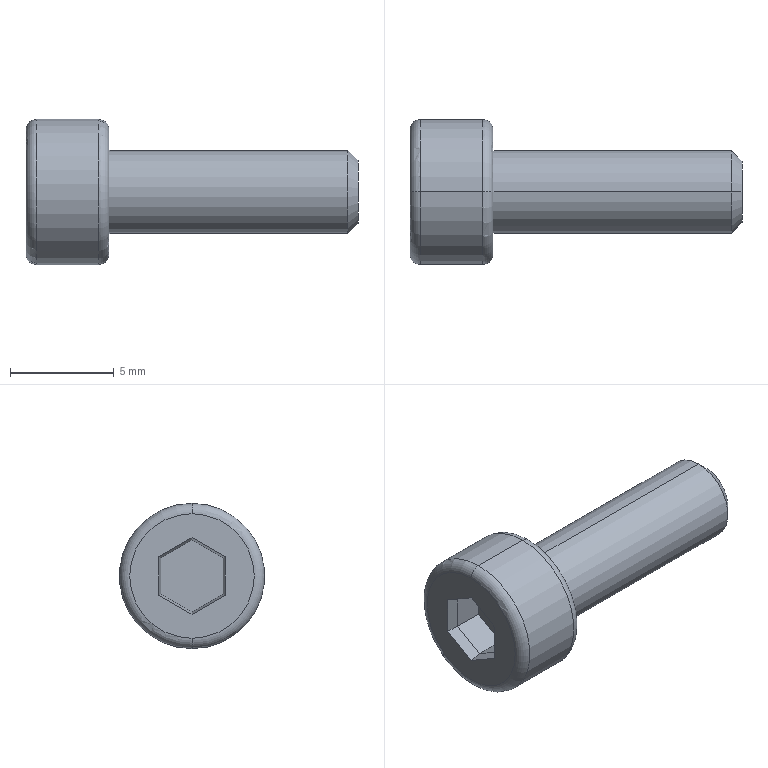Part | SolidWorks | features Chamfer 2, Fillet 1, ICE 1, Revolution 1 | 1 solid | 26 faces | box 16 x 7 x 7 mm | volume 285.121 mm3 | plane 16 | torus 4 | cylinder 4 | cone 2 | commonest cylinder face diameters 4 x2 7 x2
STEP:
#1=CARTESIAN_POINT('',(16.,0.,-1.5));
#2=VERTEX_POINT('',#1);
#3=CARTESIAN_POINT('',(16.,0.,1.5));
#4=VERTEX_POINT('',#3);
#5=CARTESIAN_POINT('',(16.,0.,0.));
#6=DIRECTION('',(1.,0.,0.));
#7=DIRECTION('',(0.,0.,1.));
#8=AXIS2_PLACEMENT_3D('',#5,#6,#7);
#9=CIRCLE('',#8,1.5);
#10=EDGE_CURVE('',#2,#4,#9,.T.);
#11=ORIENTED_EDGE('',*,*,#10,.F.);
#12=CARTESIAN_POINT('',(15.5,0.,-2.));
#13=VERTEX_POINT('',#12);
#14=CARTESIAN_POINT('',(15.5,0.,-2.));
#15=DIRECTION('',(-0.7071,0.,-0.7071));
#16=VECTOR('',#15,1000.);
#17=LINE('',#14,#16);
#18=EDGE_CURVE('',#2,#13,#17,.T.);
#19=ORIENTED_EDGE('',*,*,#18,.T.);
#20=CARTESIAN_POINT('',(15.5,0.,2.));
#21=VERTEX_POINT('',#20);
#22=CARTESIAN_POINT('',(15.5,0.,0.));
#23=DIRECTION('',(-1.,0.,0.));
#24=DIRECTION('',(0.,0.,1.));
#25=AXIS2_PLACEMENT_3D('',#22,#23,#24);
#26=CIRCLE('',#25,2.);
#27=EDGE_CURVE('',#21,#13,#26,.T.);
#28=ORIENTED_EDGE('',*,*,#27,.F.);
#29=CARTESIAN_POINT('',(15.5,0.,2.));
#30=DIRECTION('',(-0.7071,0.,0.7071));
#31=VECTOR('',#30,1000.);
#32=LINE('',#29,#31);
#33=EDGE_CURVE('',#4,#21,#32,.T.);
#34=ORIENTED_EDGE('',*,*,#33,.F.);
#35=EDGE_LOOP('',(#11,#19,#28,#34));
#36=FACE_OUTER_BOUND('',#35,.T.);
#37=CARTESIAN_POINT('',(15.5,0.,0.));
#38=DIRECTION('',(-1.,0.,0.));
#39=DIRECTION('',(0.,0.,1.));
#40=AXIS2_PLACEMENT_3D('',#37,#38,#39);
#41=CONICAL_SURFACE('',#40,2.,0.7854);
#42=ADVANCED_FACE('',(#36),#41,.T.);
#43=CARTESIAN_POINT('',(0.,0.,3.));
#44=VERTEX_POINT('',#43);
#45=CARTESIAN_POINT('',(0.,0.,-3.));
#46=VERTEX_POINT('',#45);
#47=CARTESIAN_POINT('',(0.,0.,0.));
#48=DIRECTION('',(-1.,0.,0.));
#49=DIRECTION('',(0.,0.,-1.));
#50=AXIS2_PLACEMENT_3D('',#47,#48,#49);
#51=CIRCLE('',#50,3.);
#52=EDGE_CURVE('',#44,#46,#51,.T.);
#53=ORIENTED_EDGE('',*,*,#52,.F.);
#54=CARTESIAN_POINT('',(0.5,0.,3.5));
#55=VERTEX_POINT('',#54);
#56=CARTESIAN_POINT('',(0.5,0.,3.));
#57=DIRECTION('',(0.,1.,0.));
#58=DIRECTION('',(0.,0.,1.));
#59=AXIS2_PLACEMENT_3D('',#56,#57,#58);
#60=CIRCLE('',#59,0.5);
#61=EDGE_CURVE('',#44,#55,#60,.T.);
#62=ORIENTED_EDGE('',*,*,#61,.T.);
#63=CARTESIAN_POINT('',(0.5,0.,-3.5));
#64=VERTEX_POINT('',#63);
#65=CARTESIAN_POINT('',(0.5,0.,0.));
#66=DIRECTION('',(1.,0.,0.));
#67=DIRECTION('',(0.,0.,-1.));
#68=AXIS2_PLACEMENT_3D('',#65,#66,#67);
#69=CIRCLE('',#68,3.5);
#70=EDGE_CURVE('',#64,#55,#69,.T.);
#71=ORIENTED_EDGE('',*,*,#70,.F.);
#72=CARTESIAN_POINT('',(0.5,0.,-3.));
#73=DIRECTION('',(0.,-1.,0.));
#74=DIRECTION('',(0.,0.,-1.));
#75=AXIS2_PLACEMENT_3D('',#72,#73,#74);
#76=CIRCLE('',#75,0.5);
#77=EDGE_CURVE('',#46,#64,#76,.T.);
#78=ORIENTED_EDGE('',*,*,#77,.F.);
#79=EDGE_LOOP('',(#53,#62,#71,#78));
#80=FACE_OUTER_BOUND('',#79,.T.);
#81=CARTESIAN_POINT('',(0.5,0.,0.));
#82=DIRECTION('',(1.,0.,0.));
#83=DIRECTION('',(0.,0.,-1.));
#84=AXIS2_PLACEMENT_3D('',#81,#82,#83);
#85=TOROIDAL_SURFACE('',#84,3.,0.5);
#86=ADVANCED_FACE('',(#80),#85,.T.);
#87=CARTESIAN_POINT('',(4.,0.,-3.));
#88=VERTEX_POINT('',#87);
#89=CARTESIAN_POINT('',(4.,0.,3.));
#90=VERTEX_POINT('',#89);
#91=CARTESIAN_POINT('',(4.,0.,0.));
#92=DIRECTION('',(1.,0.,0.));
#93=DIRECTION('',(0.,0.,1.));
#94=AXIS2_PLACEMENT_3D('',#91,#92,#93);
#95=CIRCLE('',#94,3.);
#96=EDGE_CURVE('',#88,#90,#95,.T.);
#97=ORIENTED_EDGE('',*,*,#96,.F.);
#98=CARTESIAN_POINT('',(3.5,0.,-3.5));
#99=VERTEX_POINT('',#98);
#100=CARTESIAN_POINT('',(3.5,0.,-3.));
#101=DIRECTION('',(0.,1.,0.));
#102=DIRECTION('',(0.,0.,1.));
#103=AXIS2_PLACEMENT_3D('',#100,#101,#102);
#104=CIRCLE('',#103,0.5);
#105=EDGE_CURVE('',#88,#99,#104,.T.);
#106=ORIENTED_EDGE('',*,*,#105,.T.);
#107=CARTESIAN_POINT('',(3.5,0.,3.5));
#108=VERTEX_POINT('',#107);
#109=CARTESIAN_POINT('',(3.5,0.,0.));
#110=DIRECTION('',(-1.,0.,0.));
#111=DIRECTION('',(0.,0.,1.));
#112=AXIS2_PLACEMENT_3D('',#109,#110,#111);
#113=CIRCLE('',#112,3.5);
#114=EDGE_CURVE('',#108,#99,#113,.T.);
#115=ORIENTED_EDGE('',*,*,#114,.F.);
#116=CARTESIAN_POINT('',(3.5,0.,3.));
#117=DIRECTION('',(0.,-1.,0.));
#118=DIRECTION('',(0.,0.,-1.));
#119=AXIS2_PLACEMENT_3D('',#116,#117,#118);
#120=CIRCLE('',#119,0.5);
#121=EDGE_CURVE('',#90,#108,#120,.T.);
#122=ORIENTED_EDGE('',*,*,#121,.F.);
#123=EDGE_LOOP('',(#97,#106,#115,#122));
#124=FACE_OUTER_BOUND('',#123,.T.);
#125=CARTESIAN_POINT('',(3.5,0.,0.));
#126=DIRECTION('',(-1.,0.,0.));
#127=DIRECTION('',(0.,0.,1.));
#128=AXIS2_PLACEMENT_3D('',#125,#126,#127);
#129=TOROIDAL_SURFACE('',#128,3.,0.5);
#130=ADVANCED_FACE('',(#124),#129,.T.);
#131=ORIENTED_EDGE('',*,*,#27,.T.);
#132=CARTESIAN_POINT('',(4.,0.,-2.));
#133=VERTEX_POINT('',#132);
#134=CARTESIAN_POINT('',(-4.709,0.,-2.));
#135=DIRECTION('',(-1.,0.,0.));
#136=VECTOR('',#135,1000.);
#137=LINE('',#134,#136);
#138=EDGE_CURVE('',#13,#133,#137,.T.);
#139=ORIENTED_EDGE('',*,*,#138,.T.);
#140=CARTESIAN_POINT('',(4.,0.,2.));
#141=VERTEX_POINT('',#140);
#142=CARTESIAN_POINT('',(4.,0.,0.));
#143=DIRECTION('',(-1.,0.,0.));
#144=DIRECTION('',(0.,0.,1.));
#145=AXIS2_PLACEMENT_3D('',#142,#143,#144);
#146=CIRCLE('',#145,2.);
#147=EDGE_CURVE('',#141,#133,#146,.T.);
#148=ORIENTED_EDGE('',*,*,#147,.F.);
#149=CARTESIAN_POINT('',(-4.709,0.,2.));
#150=DIRECTION('',(-1.,0.,0.));
#151=VECTOR('',#150,1000.);
#152=LINE('',#149,#151);
#153=EDGE_CURVE('',#21,#141,#152,.T.);
#154=ORIENTED_EDGE('',*,*,#153,.F.);
#155=EDGE_LOOP('',(#131,#139,#148,#154));
#156=FACE_OUTER_BOUND('',#155,.T.);
#157=CARTESIAN_POINT('',(-4.709,0.,0.));
#158=DIRECTION('',(-1.,0.,0.));
#159=DIRECTION('',(0.,0.,1.));
#160=AXIS2_PLACEMENT_3D('',#157,#158,#159);
#161=CYLINDRICAL_SURFACE('',#160,2.);
#162=ADVANCED_FACE('',(#156),#161,.T.);
#163=ORIENTED_EDGE('',*,*,#114,.T.);
#164=CARTESIAN_POINT('',(-4.709,0.,-3.5));
#165=DIRECTION('',(-1.,0.,0.));
#166=VECTOR('',#165,1000.);
#167=LINE('',#164,#166);
#168=EDGE_CURVE('',#99,#64,#167,.T.);
#169=ORIENTED_EDGE('',*,*,#168,.T.);
#170=ORIENTED_EDGE('',*,*,#70,.T.);
#171=CARTESIAN_POINT('',(-4.709,0.,3.5));
#172=DIRECTION('',(-1.,0.,0.));
#173=VECTOR('',#172,1000.);
#174=LINE('',#171,#173);
#175=EDGE_CURVE('',#108,#55,#174,.T.);
#176=ORIENTED_EDGE('',*,*,#175,.F.);
#177=EDGE_LOOP('',(#163,#169,#170,#176));
#178=FACE_OUTER_BOUND('',#177,.T.);
#179=CARTESIAN_POINT('',(-4.709,0.,0.));
#180=DIRECTION('',(-1.,0.,0.));
#181=DIRECTION('',(0.,0.,1.));
#182=AXIS2_PLACEMENT_3D('',#179,#180,#181);
#183=CYLINDRICAL_SURFACE('',#182,3.5);
#184=ADVANCED_FACE('',(#178),#183,.T.);
#185=CARTESIAN_POINT('',(0.,-1.6,0.9238));
#186=VERTEX_POINT('',#185);
#187=CARTESIAN_POINT('',(0.,-1.6,-0.9238));
#188=VERTEX_POINT('',#187);
#189=CARTESIAN_POINT('',(0.,-1.6,0.));
#190=DIRECTION('',(0.,0.,-1.));
#191=VECTOR('',#190,1000.);
#192=LINE('',#189,#191);
#193=EDGE_CURVE('',#186,#188,#192,.T.);
#194=ORIENTED_EDGE('',*,*,#193,.T.);
#195=CARTESIAN_POINT('',(0.,0.,-1.848));
#196=VERTEX_POINT('',#195);
#197=CARTESIAN_POINT('',(0.,-0.8,-1.386));
#198=DIRECTION('',(0.,0.866,-0.5));
#199=VECTOR('',#198,1000.);
#200=LINE('',#197,#199);
#201=EDGE_CURVE('',#188,#196,#200,.T.);
#202=ORIENTED_EDGE('',*,*,#201,.T.);
#203=CARTESIAN_POINT('',(0.,1.6,-0.9238));
#204=VERTEX_POINT('',#203);
#205=CARTESIAN_POINT('',(0.,0.8,-1.386));
#206=DIRECTION('',(0.,0.866,0.5));
#207=VECTOR('',#206,1000.);
#208=LINE('',#205,#207);
#209=EDGE_CURVE('',#196,#204,#208,.T.);
#210=ORIENTED_EDGE('',*,*,#209,.T.);
#211=CARTESIAN_POINT('',(0.,1.6,0.9238));
#212=VERTEX_POINT('',#211);
#213=CARTESIAN_POINT('',(0.,1.6,0.));
#214=DIRECTION('',(0.,0.,1.));
#215=VECTOR('',#214,1000.);
#216=LINE('',#213,#215);
#217=EDGE_CURVE('',#204,#212,#216,.T.);
#218=ORIENTED_EDGE('',*,*,#217,.T.);
#219=CARTESIAN_POINT('',(0.,0.,1.848));
#220=VERTEX_POINT('',#219);
#221=CARTESIAN_POINT('',(0.,0.8,1.386));
#222=DIRECTION('',(0.,-0.866,0.5));
#223=VECTOR('',#222,1000.);
#224=LINE('',#221,#223);
#225=EDGE_CURVE('',#212,#220,#224,.T.);
#226=ORIENTED_EDGE('',*,*,#225,.T.);
#227=CARTESIAN_POINT('',(0.,-0.8,1.386));
#228=DIRECTION('',(0.,-0.866,-0.5));
#229=VECTOR('',#228,1000.);
#230=LINE('',#227,#229);
#231=EDGE_CURVE('',#220,#186,#230,.T.);
#232=ORIENTED_EDGE('',*,*,#231,.T.);
#233=EDGE_LOOP('',(#194,#202,#210,#218,#226,#232));
#234=FACE_BOUND('',#233,.T.);
#235=CARTESIAN_POINT('',(0.,0.,0.));
#236=DIRECTION('',(-1.,0.,0.));
#237=DIRECTION('',(0.,0.,-1.));
#238=AXIS2_PLACEMENT_3D('',#235,#236,#237);
#239=CIRCLE('',#238,3.);
#240=EDGE_CURVE('',#46,#44,#239,.T.);
#241=ORIENTED_EDGE('',*,*,#240,.T.);
#242=ORIENTED_EDGE('',*,*,#52,.T.);
#243=EDGE_LOOP('',(#241,#242));
#244=FACE_OUTER_BOUND('',#243,.T.);
#245=CARTESIAN_POINT('',(0.,0.,0.));
#246=DIRECTION('',(1.,0.,0.));
#247=DIRECTION('',(0.,0.,-1.));
#248=AXIS2_PLACEMENT_3D('',#245,#246,#247);
#249=PLANE('',#248);
#250=ADVANCED_FACE('',(#234,#244),#249,.F.);
#251=ORIENTED_EDGE('',*,*,#168,.F.);
#252=CARTESIAN_POINT('',(3.5,0.,0.));
#253=DIRECTION('',(-1.,0.,0.));
#254=DIRECTION('',(0.,0.,1.));
#255=AXIS2_PLACEMENT_3D('',#252,#253,#254);
#256=CIRCLE('',#255,3.5);
#257=EDGE_CURVE('',#99,#108,#256,.T.);
#258=ORIENTED_EDGE('',*,*,#257,.T.);
#259=ORIENTED_EDGE('',*,*,#175,.T.);
#260=CARTESIAN_POINT('',(0.5,0.,0.));
#261=DIRECTION('',(1.,0.,0.));
#262=DIRECTION('',(0.,0.,-1.));
#263=AXIS2_PLACEMENT_3D('',#260,#261,#262);
#264=CIRCLE('',#263,3.5);
#265=EDGE_CURVE('',#55,#64,#264,.T.);
#266=ORIENTED_EDGE('',*,*,#265,.T.);
#267=EDGE_LOOP('',(#251,#258,#259,#266));
#268=FACE_OUTER_BOUND('',#267,.T.);
#269=CARTESIAN_POINT('',(-4.709,0.,0.));
#270=DIRECTION('',(-1.,0.,0.));
#271=DIRECTION('',(0.,0.,1.));
#272=AXIS2_PLACEMENT_3D('',#269,#270,#271);
#273=CYLINDRICAL_SURFACE('',#272,3.5);
#274=ADVANCED_FACE('',(#268),#273,.T.);
#275=CARTESIAN_POINT('',(4.,0.,0.));
#276=DIRECTION('',(1.,0.,0.));
#277=DIRECTION('',(0.,0.,1.));
#278=AXIS2_PLACEMENT_3D('',#275,#276,#277);
#279=CIRCLE('',#278,3.);
#280=EDGE_CURVE('',#90,#88,#279,.T.);
#281=ORIENTED_EDGE('',*,*,#280,.T.);
#282=ORIENTED_EDGE('',*,*,#96,.T.);
#283=EDGE_LOOP('',(#281,#282));
#284=FACE_OUTER_BOUND('',#283,.T.);
#285=ORIENTED_EDGE('',*,*,#147,.T.);
#286=CARTESIAN_POINT('',(4.,0.,0.));
#287=DIRECTION('',(-1.,0.,0.));
#288=DIRECTION('',(0.,0.,1.));
#289=AXIS2_PLACEMENT_3D('',#286,#287,#288);
#290=CIRCLE('',#289,2.);
#291=EDGE_CURVE('',#133,#141,#290,.T.);
#292=ORIENTED_EDGE('',*,*,#291,.T.);
#293=EDGE_LOOP('',(#285,#292));
#294=FACE_BOUND('',#293,.T.);
#295=CARTESIAN_POINT('',(4.,3.5,0.));
#296=DIRECTION('',(-1.,0.,0.));
#297=DIRECTION('',(0.,0.,1.));
#298=AXIS2_PLACEMENT_3D('',#295,#296,#297);
#299=PLANE('',#298);
#300=ADVANCED_FACE('',(#284,#294),#299,.F.);
#301=ORIENTED_EDGE('',*,*,#138,.F.);
#302=CARTESIAN_POINT('',(15.5,0.,0.));
#303=DIRECTION('',(-1.,0.,0.));
#304=DIRECTION('',(0.,0.,1.));
#305=AXIS2_PLACEMENT_3D('',#302,#303,#304);
#306=CIRCLE('',#305,2.);
#307=EDGE_CURVE('',#13,#21,#306,.T.);
#308=ORIENTED_EDGE('',*,*,#307,.T.);
#309=ORIENTED_EDGE('',*,*,#153,.T.);
#310=ORIENTED_EDGE('',*,*,#291,.F.);
#311=EDGE_LOOP('',(#301,#308,#309,#310));
#312=FACE_OUTER_BOUND('',#311,.T.);
#313=CARTESIAN_POINT('',(-4.709,0.,0.));
#314=DIRECTION('',(-1.,0.,0.));
#315=DIRECTION('',(0.,0.,1.));
#316=AXIS2_PLACEMENT_3D('',#313,#314,#315);
#317=CYLINDRICAL_SURFACE('',#316,2.);
#318=ADVANCED_FACE('',(#312),#317,.T.);
#319=CARTESIAN_POINT('',(16.,0.,0.));
#320=DIRECTION('',(1.,0.,0.));
#321=DIRECTION('',(0.,0.,1.));
#322=AXIS2_PLACEMENT_3D('',#319,#320,#321);
#323=CIRCLE('',#322,1.5);
#324=EDGE_CURVE('',#4,#2,#323,.T.);
#325=ORIENTED_EDGE('',*,*,#324,.T.);
#326=ORIENTED_EDGE('',*,*,#10,.T.);
#327=EDGE_LOOP('',(#325,#326));
#328=FACE_OUTER_BOUND('',#327,.T.);
#329=CARTESIAN_POINT('',(16.,2.,0.));
#330=DIRECTION('',(-1.,0.,0.));
#331=DIRECTION('',(0.,0.,1.));
#332=AXIS2_PLACEMENT_3D('',#329,#330,#331);
#333=PLANE('',#332);
#334=ADVANCED_FACE('',(#328),#333,.F.);
#335=CARTESIAN_POINT('',(2.,1.5,-0.866));
#336=VERTEX_POINT('',#335);
#337=CARTESIAN_POINT('',(0.5671,1.5,-0.866));
#338=VERTEX_POINT('',#337);
#339=CARTESIAN_POINT('',(2.,1.5,-0.866));
#340=DIRECTION('',(-1.,0.,0.));
#341=VECTOR('',#340,1000.);
#342=LINE('',#339,#341);
#343=EDGE_CURVE('',#336,#338,#342,.T.);
#344=ORIENTED_EDGE('',*,*,#343,.T.);
#345=CARTESIAN_POINT('',(0.5671,0.,-1.732));
#346=VERTEX_POINT('',#345);
#347=CARTESIAN_POINT('',(0.5671,1.5,-0.866));
#348=DIRECTION('',(0.,-0.866,-0.5));
#349=VECTOR('',#348,1000.);
#350=LINE('',#347,#349);
#351=EDGE_CURVE('',#338,#346,#350,.T.);
#352=ORIENTED_EDGE('',*,*,#351,.T.);
#353=CARTESIAN_POINT('',(2.,0.,-1.732));
#354=VERTEX_POINT('',#353);
#355=CARTESIAN_POINT('',(2.,0.,-1.732));
#356=DIRECTION('',(-1.,0.,0.));
#357=VECTOR('',#356,1000.);
#358=LINE('',#355,#357);
#359=EDGE_CURVE('',#354,#346,#358,.T.);
#360=ORIENTED_EDGE('',*,*,#359,.F.);
#361=CARTESIAN_POINT('',(2.,1.5,-0.866));
#362=DIRECTION('',(0.,-0.866,-0.5));
#363=VECTOR('',#362,1000.);
#364=LINE('',#361,#363);
#365=EDGE_CURVE('',#336,#354,#364,.T.);
#366=ORIENTED_EDGE('',*,*,#365,.F.);
#367=EDGE_LOOP('',(#344,#352,#360,#366));
#368=FACE_OUTER_BOUND('',#367,.T.);
#369=CARTESIAN_POINT('',(2.,1.5,-0.866));
#370=DIRECTION('',(0.,0.5,-0.866));
#371=DIRECTION('',(0.,0.866,0.5));
#372=AXIS2_PLACEMENT_3D('',#369,#370,#371);
#373=PLANE('',#372);
#374=ADVANCED_FACE('',(#368),#373,.F.);
#375=CARTESIAN_POINT('',(2.,1.5,0.866));
#376=VERTEX_POINT('',#375);
#377=CARTESIAN_POINT('',(0.5671,1.5,0.866));
#378=VERTEX_POINT('',#377);
#379=CARTESIAN_POINT('',(2.,1.5,0.866));
#380=DIRECTION('',(-1.,0.,0.));
#381=VECTOR('',#380,1000.);
#382=LINE('',#379,#381);
#383=EDGE_CURVE('',#376,#378,#382,.T.);
#384=ORIENTED_EDGE('',*,*,#383,.T.);
#385=CARTESIAN_POINT('',(0.5671,1.5,0.866));
#386=DIRECTION('',(0.,0.,-1.));
#387=VECTOR('',#386,1000.);
#388=LINE('',#385,#387);
#389=EDGE_CURVE('',#378,#338,#388,.T.);
#390=ORIENTED_EDGE('',*,*,#389,.T.);
#391=ORIENTED_EDGE('',*,*,#343,.F.);
#392=CARTESIAN_POINT('',(2.,1.5,0.866));
#393=DIRECTION('',(0.,0.,-1.));
#394=VECTOR('',#393,1000.);
#395=LINE('',#392,#394);
#396=EDGE_CURVE('',#376,#336,#395,.T.);
#397=ORIENTED_EDGE('',*,*,#396,.F.);
#398=EDGE_LOOP('',(#384,#390,#391,#397));
#399=FACE_OUTER_BOUND('',#398,.T.);
#400=CARTESIAN_POINT('',(2.,1.5,0.866));
#401=DIRECTION('',(0.,1.,0.));
#402=DIRECTION('',(0.,0.,1.));
#403=AXIS2_PLACEMENT_3D('',#400,#401,#402);
#404=PLANE('',#403);
#405=ADVANCED_FACE('',(#399),#404,.F.);
#406=CARTESIAN_POINT('',(2.,0.,1.732));
#407=VERTEX_POINT('',#406);
#408=CARTESIAN_POINT('',(0.5671,0.,1.732));
#409=VERTEX_POINT('',#408);
#410=CARTESIAN_POINT('',(2.,0.,1.732));
#411=DIRECTION('',(-1.,0.,0.));
#412=VECTOR('',#411,1000.);
#413=LINE('',#410,#412);
#414=EDGE_CURVE('',#407,#409,#413,.T.);
#415=ORIENTED_EDGE('',*,*,#414,.T.);
#416=CARTESIAN_POINT('',(0.5671,0.,1.732));
#417=DIRECTION('',(0.,0.866,-0.5));
#418=VECTOR('',#417,1000.);
#419=LINE('',#416,#418);
#420=EDGE_CURVE('',#409,#378,#419,.T.);
#421=ORIENTED_EDGE('',*,*,#420,.T.);
#422=ORIENTED_EDGE('',*,*,#383,.F.);
#423=CARTESIAN_POINT('',(2.,0.,1.732));
#424=DIRECTION('',(0.,0.866,-0.5));
#425=VECTOR('',#424,1000.);
#426=LINE('',#423,#425);
#427=EDGE_CURVE('',#407,#376,#426,.T.);
#428=ORIENTED_EDGE('',*,*,#427,.F.);
#429=EDGE_LOOP('',(#415,#421,#422,#428));
#430=FACE_OUTER_BOUND('',#429,.T.);
#431=CARTESIAN_POINT('',(2.,0.,1.732));
#432=DIRECTION('',(0.,0.5,0.866));
#433=DIRECTION('',(0.,-0.866,0.5));
#434=AXIS2_PLACEMENT_3D('',#431,#432,#433);
#435=PLANE('',#434);
#436=ADVANCED_FACE('',(#430),#435,.F.);
#437=CARTESIAN_POINT('',(2.,-1.5,0.866));
#438=VERTEX_POINT('',#437);
#439=CARTESIAN_POINT('',(0.5671,-1.5,0.866));
#440=VERTEX_POINT('',#439);
#441=CARTESIAN_POINT('',(2.,-1.5,0.866));
#442=DIRECTION('',(-1.,0.,0.));
#443=VECTOR('',#442,1000.);
#444=LINE('',#441,#443);
#445=EDGE_CURVE('',#438,#440,#444,.T.);
#446=ORIENTED_EDGE('',*,*,#445,.T.);
#447=CARTESIAN_POINT('',(0.5671,-1.5,0.866));
#448=DIRECTION('',(0.,0.866,0.5));
#449=VECTOR('',#448,1000.);
#450=LINE('',#447,#449);
#451=EDGE_CURVE('',#440,#409,#450,.T.);
#452=ORIENTED_EDGE('',*,*,#451,.T.);
#453=ORIENTED_EDGE('',*,*,#414,.F.);
#454=CARTESIAN_POINT('',(2.,-1.5,0.866));
#455=DIRECTION('',(0.,0.866,0.5));
#456=VECTOR('',#455,1000.);
#457=LINE('',#454,#456);
#458=EDGE_CURVE('',#438,#407,#457,.T.);
#459=ORIENTED_EDGE('',*,*,#458,.F.);
#460=EDGE_LOOP('',(#446,#452,#453,#459));
#461=FACE_OUTER_BOUND('',#460,.T.);
#462=CARTESIAN_POINT('',(2.,-1.5,0.866));
#463=DIRECTION('',(0.,-0.5,0.866));
#464=DIRECTION('',(0.,-0.866,-0.5));
#465=AXIS2_PLACEMENT_3D('',#462,#463,#464);
#466=PLANE('',#465);
#467=ADVANCED_FACE('',(#461),#466,.F.);
#468=CARTESIAN_POINT('',(2.,-1.5,-0.866));
#469=VERTEX_POINT('',#468);
#470=CARTESIAN_POINT('',(0.5671,-1.5,-0.866));
#471=VERTEX_POINT('',#470);
#472=CARTESIAN_POINT('',(2.,-1.5,-0.866));
#473=DIRECTION('',(-1.,0.,0.));
#474=VECTOR('',#473,1000.);
#475=LINE('',#472,#474);
#476=EDGE_CURVE('',#469,#471,#475,.T.);
#477=ORIENTED_EDGE('',*,*,#476,.T.);
#478=CARTESIAN_POINT('',(0.5671,-1.5,-0.866));
#479=DIRECTION('',(0.,0.,1.));
#480=VECTOR('',#479,1000.);
#481=LINE('',#478,#480);
#482=EDGE_CURVE('',#471,#440,#481,.T.);
#483=ORIENTED_EDGE('',*,*,#482,.T.);
#484=ORIENTED_EDGE('',*,*,#445,.F.);
#485=CARTESIAN_POINT('',(2.,-1.5,-0.866));
#486=DIRECTION('',(0.,0.,1.));
#487=VECTOR('',#486,1000.);
#488=LINE('',#485,#487);
#489=EDGE_CURVE('',#469,#438,#488,.T.);
#490=ORIENTED_EDGE('',*,*,#489,.F.);
#491=EDGE_LOOP('',(#477,#483,#484,#490));
#492=FACE_OUTER_BOUND('',#491,.T.);
#493=CARTESIAN_POINT('',(2.,-1.5,-0.866));
#494=DIRECTION('',(0.,-1.,0.));
#495=DIRECTION('',(0.,0.,-1.));
#496=AXIS2_PLACEMENT_3D('',#493,#494,#495);
#497=PLANE('',#496);
#498=ADVANCED_FACE('',(#492),#497,.F.);
#499=ORIENTED_EDGE('',*,*,#359,.T.);
#500=CARTESIAN_POINT('',(0.5671,0.,-1.732));
#501=DIRECTION('',(0.,-0.866,0.5));
#502=VECTOR('',#501,1000.);
#503=LINE('',#500,#502);
#504=EDGE_CURVE('',#346,#471,#503,.T.);
#505=ORIENTED_EDGE('',*,*,#504,.T.);
#506=ORIENTED_EDGE('',*,*,#476,.F.);
#507=CARTESIAN_POINT('',(2.,0.,-1.732));
#508=DIRECTION('',(0.,-0.866,0.5));
#509=VECTOR('',#508,1000.);
#510=LINE('',#507,#509);
#511=EDGE_CURVE('',#354,#469,#510,.T.);
#512=ORIENTED_EDGE('',*,*,#511,.F.);
#513=EDGE_LOOP('',(#499,#505,#506,#512));
#514=FACE_OUTER_BOUND('',#513,.T.);
#515=CARTESIAN_POINT('',(2.,0.,-1.732));
#516=DIRECTION('',(0.,-0.5,-0.866));
#517=DIRECTION('',(0.,0.866,-0.5));
#518=AXIS2_PLACEMENT_3D('',#515,#516,#517);
#519=PLANE('',#518);
#520=ADVANCED_FACE('',(#514),#519,.F.);
#521=ORIENTED_EDGE('',*,*,#365,.T.);
#522=ORIENTED_EDGE('',*,*,#511,.T.);
#523=ORIENTED_EDGE('',*,*,#489,.T.);
#524=ORIENTED_EDGE('',*,*,#458,.T.);
#525=ORIENTED_EDGE('',*,*,#427,.T.);
#526=ORIENTED_EDGE('',*,*,#396,.T.);
#527=EDGE_LOOP('',(#521,#522,#523,#524,#525,#526));
#528=FACE_OUTER_BOUND('',#527,.T.);
#529=CARTESIAN_POINT('',(2.,0.,0.));
#530=DIRECTION('',(-1.,0.,0.));
#531=DIRECTION('',(0.,0.,1.));
#532=AXIS2_PLACEMENT_3D('',#529,#530,#531);
#533=PLANE('',#532);
#534=ADVANCED_FACE('',(#528),#533,.T.);
#535=ORIENTED_EDGE('',*,*,#105,.F.);
#536=ORIENTED_EDGE('',*,*,#280,.F.);
#537=ORIENTED_EDGE('',*,*,#121,.T.);
#538=ORIENTED_EDGE('',*,*,#257,.F.);
#539=EDGE_LOOP('',(#535,#536,#537,#538));
#540=FACE_OUTER_BOUND('',#539,.T.);
#541=CARTESIAN_POINT('',(3.5,0.,0.));
#542=DIRECTION('',(-1.,0.,0.));
#543=DIRECTION('',(0.,0.,1.));
#544=AXIS2_PLACEMENT_3D('',#541,#542,#543);
#545=TOROIDAL_SURFACE('',#544,3.,0.5);
#546=ADVANCED_FACE('',(#540),#545,.T.);
#547=ORIENTED_EDGE('',*,*,#61,.F.);
#548=ORIENTED_EDGE('',*,*,#240,.F.);
#549=ORIENTED_EDGE('',*,*,#77,.T.);
#550=ORIENTED_EDGE('',*,*,#265,.F.);
#551=EDGE_LOOP('',(#547,#548,#549,#550));
#552=FACE_OUTER_BOUND('',#551,.T.);
#553=CARTESIAN_POINT('',(0.5,0.,0.));
#554=DIRECTION('',(1.,0.,0.));
#555=DIRECTION('',(0.,0.,-1.));
#556=AXIS2_PLACEMENT_3D('',#553,#554,#555);
#557=TOROIDAL_SURFACE('',#556,3.,0.5);
#558=ADVANCED_FACE('',(#552),#557,.T.);
#559=CARTESIAN_POINT('',(0.7364,0.,1.698));
#560=DIRECTION('',(0.9799,0.,-0.1995));
#561=VECTOR('',#560,1000.);
#562=LINE('',#559,#561);
#563=EDGE_CURVE('',#220,#409,#562,.T.);
#564=ORIENTED_EDGE('',*,*,#563,.F.);
#565=ORIENTED_EDGE('',*,*,#225,.F.);
#566=CARTESIAN_POINT('',(0.7364,1.47,0.8488));
#567=DIRECTION('',(-0.9799,0.1728,0.09976));
#568=VECTOR('',#567,1000.);
#569=LINE('',#566,#568);
#570=EDGE_CURVE('',#378,#212,#569,.T.);
#571=ORIENTED_EDGE('',*,*,#570,.F.);
#572=ORIENTED_EDGE('',*,*,#420,.F.);
#573=EDGE_LOOP('',(#564,#565,#571,#572));
#574=FACE_OUTER_BOUND('',#573,.T.);
#575=CARTESIAN_POINT('',(0.5671,0.,1.732));
#576=DIRECTION('',(0.1736,0.4924,0.8529));
#577=DIRECTION('',(0.,0.866,-0.5));
#578=AXIS2_PLACEMENT_3D('',#575,#576,#577);
#579=PLANE('',#578);
#580=ADVANCED_FACE('',(#574),#579,.F.);
#581=ORIENTED_EDGE('',*,*,#570,.T.);
#582=ORIENTED_EDGE('',*,*,#217,.F.);
#583=CARTESIAN_POINT('',(0.7364,1.47,-0.8488));
#584=DIRECTION('',(-0.9799,0.1728,-0.09976));
#585=VECTOR('',#584,1000.);
#586=LINE('',#583,#585);
#587=EDGE_CURVE('',#338,#204,#586,.T.);
#588=ORIENTED_EDGE('',*,*,#587,.F.);
#589=ORIENTED_EDGE('',*,*,#389,.F.);
#590=EDGE_LOOP('',(#581,#582,#588,#589));
#591=FACE_OUTER_BOUND('',#590,.T.);
#592=CARTESIAN_POINT('',(0.5671,1.5,0.866));
#593=DIRECTION('',(0.1736,0.9848,0.));
#594=DIRECTION('',(0.,0.,-1.));
#595=AXIS2_PLACEMENT_3D('',#592,#593,#594);
#596=PLANE('',#595);
#597=ADVANCED_FACE('',(#591),#596,.F.);
#598=ORIENTED_EDGE('',*,*,#563,.T.);
#599=ORIENTED_EDGE('',*,*,#451,.F.);
#600=CARTESIAN_POINT('',(0.7364,-1.47,0.8488));
#601=DIRECTION('',(0.9799,0.1728,-0.09976));
#602=VECTOR('',#601,1000.);
#603=LINE('',#600,#602);
#604=EDGE_CURVE('',#186,#440,#603,.T.);
#605=ORIENTED_EDGE('',*,*,#604,.F.);
#606=ORIENTED_EDGE('',*,*,#231,.F.);
#607=EDGE_LOOP('',(#598,#599,#605,#606));
#608=FACE_OUTER_BOUND('',#607,.T.);
#609=CARTESIAN_POINT('',(0.5671,-1.5,0.866));
#610=DIRECTION('',(0.1736,-0.4924,0.8529));
#611=DIRECTION('',(0.,0.866,0.5));
#612=AXIS2_PLACEMENT_3D('',#609,#610,#611);
#613=PLANE('',#612);
#614=ADVANCED_FACE('',(#608),#613,.F.);
#615=ORIENTED_EDGE('',*,*,#587,.T.);
#616=ORIENTED_EDGE('',*,*,#209,.F.);
#617=CARTESIAN_POINT('',(0.5671,0.,-1.732));
#618=DIRECTION('',(-0.9799,0.,-0.1995));
#619=VECTOR('',#618,1000.);
#620=LINE('',#617,#619);
#621=EDGE_CURVE('',#346,#196,#620,.T.);
#622=ORIENTED_EDGE('',*,*,#621,.F.);
#623=ORIENTED_EDGE('',*,*,#351,.F.);
#624=EDGE_LOOP('',(#615,#616,#622,#623));
#625=FACE_OUTER_BOUND('',#624,.T.);
#626=CARTESIAN_POINT('',(0.5671,1.5,-0.866));
#627=DIRECTION('',(0.1736,0.4924,-0.8529));
#628=DIRECTION('',(0.,-0.866,-0.5));
#629=AXIS2_PLACEMENT_3D('',#626,#627,#628);
#630=PLANE('',#629);
#631=ADVANCED_FACE('',(#625),#630,.F.);
#632=ORIENTED_EDGE('',*,*,#604,.T.);
#633=ORIENTED_EDGE('',*,*,#482,.F.);
#634=CARTESIAN_POINT('',(0.7364,-1.47,-0.8488));
#635=DIRECTION('',(0.9799,0.1728,0.09976));
#636=VECTOR('',#635,1000.);
#637=LINE('',#634,#636);
#638=EDGE_CURVE('',#188,#471,#637,.T.);
#639=ORIENTED_EDGE('',*,*,#638,.F.);
#640=ORIENTED_EDGE('',*,*,#193,.F.);
#641=EDGE_LOOP('',(#632,#633,#639,#640));
#642=FACE_OUTER_BOUND('',#641,.T.);
#643=CARTESIAN_POINT('',(0.5671,-1.5,-0.866));
#644=DIRECTION('',(0.1736,-0.9848,0.));
#645=DIRECTION('',(0.,0.,1.));
#646=AXIS2_PLACEMENT_3D('',#643,#644,#645);
#647=PLANE('',#646);
#648=ADVANCED_FACE('',(#642),#647,.F.);
#649=ORIENTED_EDGE('',*,*,#621,.T.);
#650=ORIENTED_EDGE('',*,*,#201,.F.);
#651=ORIENTED_EDGE('',*,*,#638,.T.);
#652=ORIENTED_EDGE('',*,*,#504,.F.);
#653=EDGE_LOOP('',(#649,#650,#651,#652));
#654=FACE_OUTER_BOUND('',#653,.T.);
#655=CARTESIAN_POINT('',(0.5671,0.,-1.732));
#656=DIRECTION('',(0.1736,-0.4924,-0.8529));
#657=DIRECTION('',(0.,-0.866,0.5));
#658=AXIS2_PLACEMENT_3D('',#655,#656,#657);
#659=PLANE('',#658);
#660=ADVANCED_FACE('',(#654),#659,.F.);
#661=ORIENTED_EDGE('',*,*,#18,.F.);
#662=ORIENTED_EDGE('',*,*,#324,.F.);
#663=ORIENTED_EDGE('',*,*,#33,.T.);
#664=ORIENTED_EDGE('',*,*,#307,.F.);
#665=EDGE_LOOP('',(#661,#662,#663,#664));
#666=FACE_OUTER_BOUND('',#665,.T.);
#667=CARTESIAN_POINT('',(15.5,0.,0.));
#668=DIRECTION('',(-1.,0.,0.));
#669=DIRECTION('',(0.,0.,1.));
#670=AXIS2_PLACEMENT_3D('',#667,#668,#669);
#671=CONICAL_SURFACE('',#670,2.,0.7854);
#672=ADVANCED_FACE('',(#666),#671,.T.);
#673=CLOSED_SHELL('',(#42,#86,#130,#162,#184,#250,#274,#300,#318,#334,#374,#405,#436,#467,#498,#520,#534,#546,#558,#580,#597,#614,#631,#648,#660,#672));
#674=MANIFOLD_SOLID_BREP('',#673);
#675=CARTESIAN_POINT('',(0.,0.,0.));
#676=DIRECTION('',(0.,0.,1.));
#677=DIRECTION('',(1.,0.,0.));
#678=AXIS2_PLACEMENT_3D('',#675,#676,#677);
#679=(LENGTH_UNIT()NAMED_UNIT(*)SI_UNIT(.MILLI.,.METRE.));
#680=UNCERTAINTY_MEASURE_WITH_UNIT(LENGTH_MEASURE(0.00001),#679,'','');
#681=(NAMED_UNIT(*)PLANE_ANGLE_UNIT()SI_UNIT($,.RADIAN.));
#682=(NAMED_UNIT(*)SI_UNIT($,.STERADIAN.)SOLID_ANGLE_UNIT());
#683=(GEOMETRIC_REPRESENTATION_CONTEXT(3)GLOBAL_UNCERTAINTY_ASSIGNED_CONTEXT((#680))GLOBAL_UNIT_ASSIGNED_CONTEXT((#679,#681,#682))REPRESENTATION_CONTEXT('',''));
#684=ADVANCED_BREP_SHAPE_REPRESENTATION('',(#674,#678),#683);